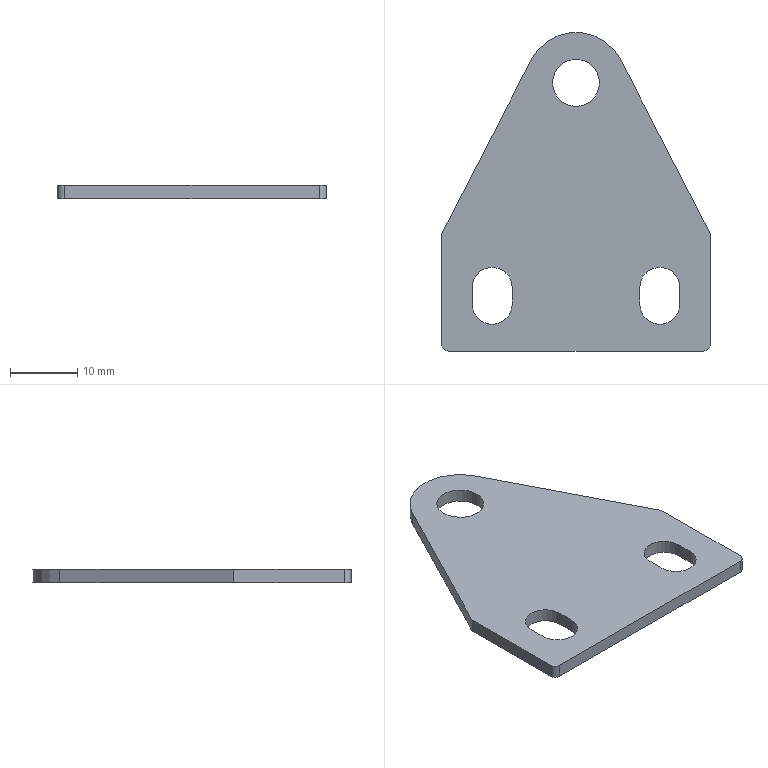Part | STEP file | LE-MX-A-P1_PN_0007 | 1 solid | 20 faces | box 40 x 47.5 x 2 mm | volume 2610 mm3 | plane 11 | cylinder 9 | commonest cylinder face diameters 6 x4 2 x2 7 x2 15 x1
STEP:
#1=CARTESIAN_POINT('',(-3.5,40.,2.));
#2=VERTEX_POINT('',#1);
#3=CARTESIAN_POINT('',(3.5,40.,2.));
#4=VERTEX_POINT('',#3);
#5=CARTESIAN_POINT('',(0.,40.,2.));
#6=DIRECTION('',(0.,0.,1.));
#7=DIRECTION('',(-1.,0.,0.));
#8=AXIS2_PLACEMENT_3D('',#5,#6,#7);
#9=CIRCLE('',#8,3.5);
#10=EDGE_CURVE('',#2,#4,#9,.T.);
#11=ORIENTED_EDGE('',*,*,#10,.T.);
#12=CARTESIAN_POINT('',(3.5,40.,0.));
#13=VERTEX_POINT('',#12);
#14=CARTESIAN_POINT('',(3.5,40.,2.));
#15=DIRECTION('',(0.,0.,-1.));
#16=VECTOR('',#15,1000.);
#17=LINE('',#14,#16);
#18=EDGE_CURVE('',#4,#13,#17,.T.);
#19=ORIENTED_EDGE('',*,*,#18,.T.);
#20=CARTESIAN_POINT('',(-3.5,40.,0.));
#21=VERTEX_POINT('',#20);
#22=CARTESIAN_POINT('',(0.,40.,0.));
#23=DIRECTION('',(0.,0.,1.));
#24=DIRECTION('',(-1.,0.,0.));
#25=AXIS2_PLACEMENT_3D('',#22,#23,#24);
#26=CIRCLE('',#25,3.5);
#27=EDGE_CURVE('',#21,#13,#26,.T.);
#28=ORIENTED_EDGE('',*,*,#27,.F.);
#29=CARTESIAN_POINT('',(-3.5,40.,2.));
#30=DIRECTION('',(0.,0.,-1.));
#31=VECTOR('',#30,1000.);
#32=LINE('',#29,#31);
#33=EDGE_CURVE('',#2,#21,#32,.T.);
#34=ORIENTED_EDGE('',*,*,#33,.F.);
#35=EDGE_LOOP('',(#11,#19,#28,#34));
#36=FACE_OUTER_BOUND('',#35,.T.);
#37=CARTESIAN_POINT('',(0.,40.,2.));
#38=DIRECTION('',(0.,0.,-1.));
#39=DIRECTION('',(-1.,0.,0.));
#40=AXIS2_PLACEMENT_3D('',#37,#38,#39);
#41=CYLINDRICAL_SURFACE('',#40,3.5);
#42=ADVANCED_FACE('',(#36),#41,.F.);
#43=CARTESIAN_POINT('',(-20.,17.5,2.));
#44=VERTEX_POINT('',#43);
#45=CARTESIAN_POINT('',(-6.67,43.429,2.));
#46=VERTEX_POINT('',#45);
#47=CARTESIAN_POINT('',(-20.,17.5,2.));
#48=DIRECTION('',(0.4572,0.8894,0.));
#49=VECTOR('',#48,1000.);
#50=LINE('',#47,#49);
#51=EDGE_CURVE('',#44,#46,#50,.T.);
#52=ORIENTED_EDGE('',*,*,#51,.F.);
#53=CARTESIAN_POINT('',(-20.,1.,2.));
#54=VERTEX_POINT('',#53);
#55=CARTESIAN_POINT('',(-20.,40.,2.));
#56=DIRECTION('',(0.,1.,0.));
#57=VECTOR('',#56,1000.);
#58=LINE('',#55,#57);
#59=EDGE_CURVE('',#54,#44,#58,.T.);
#60=ORIENTED_EDGE('',*,*,#59,.F.);
#61=CARTESIAN_POINT('',(-19.,0.,2.));
#62=VERTEX_POINT('',#61);
#63=CARTESIAN_POINT('',(-19.,1.,2.));
#64=DIRECTION('',(0.,0.,-1.));
#65=DIRECTION('',(-1.,0.,0.));
#66=AXIS2_PLACEMENT_3D('',#63,#64,#65);
#67=CIRCLE('',#66,1.);
#68=EDGE_CURVE('',#62,#54,#67,.T.);
#69=ORIENTED_EDGE('',*,*,#68,.F.);
#70=CARTESIAN_POINT('',(19.,0.,2.));
#71=VERTEX_POINT('',#70);
#72=CARTESIAN_POINT('',(0.,0.,2.));
#73=DIRECTION('',(-1.,0.,0.));
#74=VECTOR('',#73,1000.);
#75=LINE('',#72,#74);
#76=EDGE_CURVE('',#71,#62,#75,.T.);
#77=ORIENTED_EDGE('',*,*,#76,.F.);
#78=CARTESIAN_POINT('',(20.,1.,2.));
#79=VERTEX_POINT('',#78);
#80=CARTESIAN_POINT('',(19.,1.,2.));
#81=DIRECTION('',(0.,0.,-1.));
#82=DIRECTION('',(-1.,0.,0.));
#83=AXIS2_PLACEMENT_3D('',#80,#81,#82);
#84=CIRCLE('',#83,1.);
#85=EDGE_CURVE('',#79,#71,#84,.T.);
#86=ORIENTED_EDGE('',*,*,#85,.F.);
#87=CARTESIAN_POINT('',(20.,17.5,2.));
#88=VERTEX_POINT('',#87);
#89=CARTESIAN_POINT('',(20.,40.,2.));
#90=DIRECTION('',(0.,-1.,0.));
#91=VECTOR('',#90,1000.);
#92=LINE('',#89,#91);
#93=EDGE_CURVE('',#88,#79,#92,.T.);
#94=ORIENTED_EDGE('',*,*,#93,.F.);
#95=CARTESIAN_POINT('',(6.67,43.429,2.));
#96=VERTEX_POINT('',#95);
#97=CARTESIAN_POINT('',(6.67,43.429,2.));
#98=DIRECTION('',(0.4572,-0.8894,0.));
#99=VECTOR('',#98,1000.);
#100=LINE('',#97,#99);
#101=EDGE_CURVE('',#96,#88,#100,.T.);
#102=ORIENTED_EDGE('',*,*,#101,.F.);
#103=CARTESIAN_POINT('',(0.,40.,2.));
#104=DIRECTION('',(0.,0.,-1.));
#105=DIRECTION('',(-1.,0.,0.));
#106=AXIS2_PLACEMENT_3D('',#103,#104,#105);
#107=CIRCLE('',#106,7.5);
#108=EDGE_CURVE('',#46,#96,#107,.T.);
#109=ORIENTED_EDGE('',*,*,#108,.F.);
#110=EDGE_LOOP('',(#52,#60,#69,#77,#86,#94,#102,#109));
#111=FACE_OUTER_BOUND('',#110,.T.);
#112=CARTESIAN_POINT('',(15.5,9.5,2.));
#113=VERTEX_POINT('',#112);
#114=CARTESIAN_POINT('',(9.5,9.5,2.));
#115=VERTEX_POINT('',#114);
#116=CARTESIAN_POINT('',(12.5,9.5,2.));
#117=DIRECTION('',(0.,0.,1.));
#118=DIRECTION('',(-1.,0.,0.));
#119=AXIS2_PLACEMENT_3D('',#116,#117,#118);
#120=CIRCLE('',#119,3.);
#121=EDGE_CURVE('',#113,#115,#120,.T.);
#122=ORIENTED_EDGE('',*,*,#121,.F.);
#123=CARTESIAN_POINT('',(15.5,7.,2.));
#124=VERTEX_POINT('',#123);
#125=CARTESIAN_POINT('',(15.5,40.,2.));
#126=DIRECTION('',(0.,1.,0.));
#127=VECTOR('',#126,1000.);
#128=LINE('',#125,#127);
#129=EDGE_CURVE('',#124,#113,#128,.T.);
#130=ORIENTED_EDGE('',*,*,#129,.F.);
#131=CARTESIAN_POINT('',(9.5,7.,2.));
#132=VERTEX_POINT('',#131);
#133=CARTESIAN_POINT('',(12.5,7.,2.));
#134=DIRECTION('',(0.,0.,1.));
#135=DIRECTION('',(-1.,0.,0.));
#136=AXIS2_PLACEMENT_3D('',#133,#134,#135);
#137=CIRCLE('',#136,3.);
#138=EDGE_CURVE('',#132,#124,#137,.T.);
#139=ORIENTED_EDGE('',*,*,#138,.F.);
#140=CARTESIAN_POINT('',(9.5,40.,2.));
#141=DIRECTION('',(0.,-1.,0.));
#142=VECTOR('',#141,1000.);
#143=LINE('',#140,#142);
#144=EDGE_CURVE('',#115,#132,#143,.T.);
#145=ORIENTED_EDGE('',*,*,#144,.F.);
#146=EDGE_LOOP('',(#122,#130,#139,#145));
#147=FACE_BOUND('',#146,.T.);
#148=ORIENTED_EDGE('',*,*,#10,.F.);
#149=CARTESIAN_POINT('',(0.,40.,2.));
#150=DIRECTION('',(0.,0.,1.));
#151=DIRECTION('',(-1.,0.,0.));
#152=AXIS2_PLACEMENT_3D('',#149,#150,#151);
#153=CIRCLE('',#152,3.5);
#154=EDGE_CURVE('',#4,#2,#153,.T.);
#155=ORIENTED_EDGE('',*,*,#154,.F.);
#156=EDGE_LOOP('',(#148,#155));
#157=FACE_BOUND('',#156,.T.);
#158=CARTESIAN_POINT('',(-9.5,9.5,2.));
#159=VERTEX_POINT('',#158);
#160=CARTESIAN_POINT('',(-15.5,9.5,2.));
#161=VERTEX_POINT('',#160);
#162=CARTESIAN_POINT('',(-12.5,9.5,2.));
#163=DIRECTION('',(0.,0.,1.));
#164=DIRECTION('',(-1.,0.,0.));
#165=AXIS2_PLACEMENT_3D('',#162,#163,#164);
#166=CIRCLE('',#165,3.);
#167=EDGE_CURVE('',#159,#161,#166,.T.);
#168=ORIENTED_EDGE('',*,*,#167,.F.);
#169=CARTESIAN_POINT('',(-9.5,7.,2.));
#170=VERTEX_POINT('',#169);
#171=CARTESIAN_POINT('',(-9.5,40.,2.));
#172=DIRECTION('',(0.,1.,0.));
#173=VECTOR('',#172,1000.);
#174=LINE('',#171,#173);
#175=EDGE_CURVE('',#170,#159,#174,.T.);
#176=ORIENTED_EDGE('',*,*,#175,.F.);
#177=CARTESIAN_POINT('',(-15.5,7.,2.));
#178=VERTEX_POINT('',#177);
#179=CARTESIAN_POINT('',(-12.5,7.,2.));
#180=DIRECTION('',(0.,0.,1.));
#181=DIRECTION('',(-1.,0.,0.));
#182=AXIS2_PLACEMENT_3D('',#179,#180,#181);
#183=CIRCLE('',#182,3.);
#184=EDGE_CURVE('',#178,#170,#183,.T.);
#185=ORIENTED_EDGE('',*,*,#184,.F.);
#186=CARTESIAN_POINT('',(-15.5,40.,2.));
#187=DIRECTION('',(0.,-1.,0.));
#188=VECTOR('',#187,1000.);
#189=LINE('',#186,#188);
#190=EDGE_CURVE('',#161,#178,#189,.T.);
#191=ORIENTED_EDGE('',*,*,#190,.F.);
#192=EDGE_LOOP('',(#168,#176,#185,#191));
#193=FACE_BOUND('',#192,.T.);
#194=CARTESIAN_POINT('',(0.,40.,2.));
#195=DIRECTION('',(0.,0.,-1.));
#196=DIRECTION('',(-1.,0.,0.));
#197=AXIS2_PLACEMENT_3D('',#194,#195,#196);
#198=PLANE('',#197);
#199=ADVANCED_FACE('',(#111,#147,#157,#193),#198,.F.);
#200=ORIENTED_EDGE('',*,*,#108,.T.);
#201=CARTESIAN_POINT('',(6.67,43.429,0.));
#202=VERTEX_POINT('',#201);
#203=CARTESIAN_POINT('',(6.67,43.429,2.));
#204=DIRECTION('',(0.,0.,-1.));
#205=VECTOR('',#204,1000.);
#206=LINE('',#203,#205);
#207=EDGE_CURVE('',#96,#202,#206,.T.);
#208=ORIENTED_EDGE('',*,*,#207,.T.);
#209=CARTESIAN_POINT('',(-6.67,43.429,0.));
#210=VERTEX_POINT('',#209);
#211=CARTESIAN_POINT('',(0.,40.,0.));
#212=DIRECTION('',(0.,0.,1.));
#213=DIRECTION('',(-1.,0.,0.));
#214=AXIS2_PLACEMENT_3D('',#211,#212,#213);
#215=CIRCLE('',#214,7.5);
#216=EDGE_CURVE('',#202,#210,#215,.T.);
#217=ORIENTED_EDGE('',*,*,#216,.T.);
#218=CARTESIAN_POINT('',(-6.67,43.429,2.));
#219=DIRECTION('',(0.,0.,1.));
#220=VECTOR('',#219,1000.);
#221=LINE('',#218,#220);
#222=EDGE_CURVE('',#210,#46,#221,.T.);
#223=ORIENTED_EDGE('',*,*,#222,.T.);
#224=EDGE_LOOP('',(#200,#208,#217,#223));
#225=FACE_OUTER_BOUND('',#224,.T.);
#226=CARTESIAN_POINT('',(0.,40.,2.));
#227=DIRECTION('',(0.,0.,-1.));
#228=DIRECTION('',(-1.,0.,0.));
#229=AXIS2_PLACEMENT_3D('',#226,#227,#228);
#230=CYLINDRICAL_SURFACE('',#229,7.5);
#231=ADVANCED_FACE('',(#225),#230,.T.);
#232=ORIENTED_EDGE('',*,*,#51,.T.);
#233=ORIENTED_EDGE('',*,*,#222,.F.);
#234=CARTESIAN_POINT('',(-20.,17.5,0.));
#235=VERTEX_POINT('',#234);
#236=CARTESIAN_POINT('',(-20.,17.5,0.));
#237=DIRECTION('',(-0.4572,-0.8894,0.));
#238=VECTOR('',#237,1000.);
#239=LINE('',#236,#238);
#240=EDGE_CURVE('',#210,#235,#239,.T.);
#241=ORIENTED_EDGE('',*,*,#240,.T.);
#242=CARTESIAN_POINT('',(-20.,17.5,2.));
#243=DIRECTION('',(0.,0.,1.));
#244=VECTOR('',#243,1000.);
#245=LINE('',#242,#244);
#246=EDGE_CURVE('',#235,#44,#245,.T.);
#247=ORIENTED_EDGE('',*,*,#246,.T.);
#248=EDGE_LOOP('',(#232,#233,#241,#247));
#249=FACE_OUTER_BOUND('',#248,.T.);
#250=CARTESIAN_POINT('',(-20.,17.5,2.));
#251=DIRECTION('',(-0.8894,0.4572,0.));
#252=DIRECTION('',(-0.4572,-0.8894,0.));
#253=AXIS2_PLACEMENT_3D('',#250,#251,#252);
#254=PLANE('',#253);
#255=ADVANCED_FACE('',(#249),#254,.T.);
#256=ORIENTED_EDGE('',*,*,#59,.T.);
#257=ORIENTED_EDGE('',*,*,#246,.F.);
#258=CARTESIAN_POINT('',(-20.,1.,0.));
#259=VERTEX_POINT('',#258);
#260=CARTESIAN_POINT('',(-20.,1.,0.));
#261=DIRECTION('',(0.,-1.,0.));
#262=VECTOR('',#261,1000.);
#263=LINE('',#260,#262);
#264=EDGE_CURVE('',#235,#259,#263,.T.);
#265=ORIENTED_EDGE('',*,*,#264,.T.);
#266=CARTESIAN_POINT('',(-20.,1.,2.));
#267=DIRECTION('',(0.,0.,1.));
#268=VECTOR('',#267,1000.);
#269=LINE('',#266,#268);
#270=EDGE_CURVE('',#259,#54,#269,.T.);
#271=ORIENTED_EDGE('',*,*,#270,.T.);
#272=EDGE_LOOP('',(#256,#257,#265,#271));
#273=FACE_OUTER_BOUND('',#272,.T.);
#274=CARTESIAN_POINT('',(-20.,1.,2.));
#275=DIRECTION('',(-1.,0.,0.));
#276=DIRECTION('',(0.,0.,1.));
#277=AXIS2_PLACEMENT_3D('',#274,#275,#276);
#278=PLANE('',#277);
#279=ADVANCED_FACE('',(#273),#278,.T.);
#280=ORIENTED_EDGE('',*,*,#76,.T.);
#281=CARTESIAN_POINT('',(-19.,0.,0.));
#282=VERTEX_POINT('',#281);
#283=CARTESIAN_POINT('',(-19.,0.,2.));
#284=DIRECTION('',(0.,0.,-1.));
#285=VECTOR('',#284,1000.);
#286=LINE('',#283,#285);
#287=EDGE_CURVE('',#62,#282,#286,.T.);
#288=ORIENTED_EDGE('',*,*,#287,.T.);
#289=CARTESIAN_POINT('',(19.,0.,0.));
#290=VERTEX_POINT('',#289);
#291=CARTESIAN_POINT('',(19.,0.,0.));
#292=DIRECTION('',(1.,0.,0.));
#293=VECTOR('',#292,1000.);
#294=LINE('',#291,#293);
#295=EDGE_CURVE('',#282,#290,#294,.T.);
#296=ORIENTED_EDGE('',*,*,#295,.T.);
#297=CARTESIAN_POINT('',(19.,0.,2.));
#298=DIRECTION('',(0.,0.,1.));
#299=VECTOR('',#298,1000.);
#300=LINE('',#297,#299);
#301=EDGE_CURVE('',#290,#71,#300,.T.);
#302=ORIENTED_EDGE('',*,*,#301,.T.);
#303=EDGE_LOOP('',(#280,#288,#296,#302));
#304=FACE_OUTER_BOUND('',#303,.T.);
#305=CARTESIAN_POINT('',(19.,0.,2.));
#306=DIRECTION('',(0.,-1.,0.));
#307=DIRECTION('',(1.,0.,0.));
#308=AXIS2_PLACEMENT_3D('',#305,#306,#307);
#309=PLANE('',#308);
#310=ADVANCED_FACE('',(#304),#309,.T.);
#311=ORIENTED_EDGE('',*,*,#93,.T.);
#312=CARTESIAN_POINT('',(20.,1.,0.));
#313=VERTEX_POINT('',#312);
#314=CARTESIAN_POINT('',(20.,1.,2.));
#315=DIRECTION('',(0.,0.,-1.));
#316=VECTOR('',#315,1000.);
#317=LINE('',#314,#316);
#318=EDGE_CURVE('',#79,#313,#317,.T.);
#319=ORIENTED_EDGE('',*,*,#318,.T.);
#320=CARTESIAN_POINT('',(20.,17.5,0.));
#321=VERTEX_POINT('',#320);
#322=CARTESIAN_POINT('',(20.,17.5,0.));
#323=DIRECTION('',(0.,1.,0.));
#324=VECTOR('',#323,1000.);
#325=LINE('',#322,#324);
#326=EDGE_CURVE('',#313,#321,#325,.T.);
#327=ORIENTED_EDGE('',*,*,#326,.T.);
#328=CARTESIAN_POINT('',(20.,17.5,2.));
#329=DIRECTION('',(0.,0.,1.));
#330=VECTOR('',#329,1000.);
#331=LINE('',#328,#330);
#332=EDGE_CURVE('',#321,#88,#331,.T.);
#333=ORIENTED_EDGE('',*,*,#332,.T.);
#334=EDGE_LOOP('',(#311,#319,#327,#333));
#335=FACE_OUTER_BOUND('',#334,.T.);
#336=CARTESIAN_POINT('',(20.,17.5,2.));
#337=DIRECTION('',(1.,0.,0.));
#338=DIRECTION('',(0.,0.,-1.));
#339=AXIS2_PLACEMENT_3D('',#336,#337,#338);
#340=PLANE('',#339);
#341=ADVANCED_FACE('',(#335),#340,.T.);
#342=ORIENTED_EDGE('',*,*,#101,.T.);
#343=ORIENTED_EDGE('',*,*,#332,.F.);
#344=CARTESIAN_POINT('',(6.67,43.429,0.));
#345=DIRECTION('',(-0.4572,0.8894,0.));
#346=VECTOR('',#345,1000.);
#347=LINE('',#344,#346);
#348=EDGE_CURVE('',#321,#202,#347,.T.);
#349=ORIENTED_EDGE('',*,*,#348,.T.);
#350=ORIENTED_EDGE('',*,*,#207,.F.);
#351=EDGE_LOOP('',(#342,#343,#349,#350));
#352=FACE_OUTER_BOUND('',#351,.T.);
#353=CARTESIAN_POINT('',(6.67,43.429,2.));
#354=DIRECTION('',(0.8894,0.4572,0.));
#355=DIRECTION('',(-0.4572,0.8894,0.));
#356=AXIS2_PLACEMENT_3D('',#353,#354,#355);
#357=PLANE('',#356);
#358=ADVANCED_FACE('',(#352),#357,.T.);
#359=CARTESIAN_POINT('',(9.5,9.5,0.));
#360=VERTEX_POINT('',#359);
#361=CARTESIAN_POINT('',(9.5,9.5,2.));
#362=DIRECTION('',(0.,0.,-1.));
#363=VECTOR('',#362,1000.);
#364=LINE('',#361,#363);
#365=EDGE_CURVE('',#115,#360,#364,.T.);
#366=ORIENTED_EDGE('',*,*,#365,.F.);
#367=ORIENTED_EDGE('',*,*,#144,.T.);
#368=CARTESIAN_POINT('',(9.5,7.,0.));
#369=VERTEX_POINT('',#368);
#370=CARTESIAN_POINT('',(9.5,7.,2.));
#371=DIRECTION('',(0.,0.,1.));
#372=VECTOR('',#371,1000.);
#373=LINE('',#370,#372);
#374=EDGE_CURVE('',#369,#132,#373,.T.);
#375=ORIENTED_EDGE('',*,*,#374,.F.);
#376=CARTESIAN_POINT('',(9.5,9.5,0.));
#377=DIRECTION('',(0.,-1.,0.));
#378=VECTOR('',#377,1000.);
#379=LINE('',#376,#378);
#380=EDGE_CURVE('',#360,#369,#379,.T.);
#381=ORIENTED_EDGE('',*,*,#380,.F.);
#382=EDGE_LOOP('',(#366,#367,#375,#381));
#383=FACE_OUTER_BOUND('',#382,.T.);
#384=CARTESIAN_POINT('',(9.5,9.5,2.));
#385=DIRECTION('',(-1.,0.,0.));
#386=DIRECTION('',(0.,-1.,0.));
#387=AXIS2_PLACEMENT_3D('',#384,#385,#386);
#388=PLANE('',#387);
#389=ADVANCED_FACE('',(#383),#388,.F.);
#390=CARTESIAN_POINT('',(15.5,9.5,0.));
#391=VERTEX_POINT('',#390);
#392=CARTESIAN_POINT('',(15.5,9.5,2.));
#393=DIRECTION('',(0.,0.,-1.));
#394=VECTOR('',#393,1000.);
#395=LINE('',#392,#394);
#396=EDGE_CURVE('',#113,#391,#395,.T.);
#397=ORIENTED_EDGE('',*,*,#396,.F.);
#398=ORIENTED_EDGE('',*,*,#121,.T.);
#399=ORIENTED_EDGE('',*,*,#365,.T.);
#400=CARTESIAN_POINT('',(12.5,9.5,0.));
#401=DIRECTION('',(0.,0.,1.));
#402=DIRECTION('',(-1.,0.,0.));
#403=AXIS2_PLACEMENT_3D('',#400,#401,#402);
#404=CIRCLE('',#403,3.);
#405=EDGE_CURVE('',#391,#360,#404,.T.);
#406=ORIENTED_EDGE('',*,*,#405,.F.);
#407=EDGE_LOOP('',(#397,#398,#399,#406));
#408=FACE_OUTER_BOUND('',#407,.T.);
#409=CARTESIAN_POINT('',(12.5,9.5,2.));
#410=DIRECTION('',(0.,0.,-1.));
#411=DIRECTION('',(-1.,0.,0.));
#412=AXIS2_PLACEMENT_3D('',#409,#410,#411);
#413=CYLINDRICAL_SURFACE('',#412,3.);
#414=ADVANCED_FACE('',(#408),#413,.F.);
#415=CARTESIAN_POINT('',(15.5,7.,0.));
#416=VERTEX_POINT('',#415);
#417=CARTESIAN_POINT('',(15.5,7.,2.));
#418=DIRECTION('',(0.,0.,-1.));
#419=VECTOR('',#418,1000.);
#420=LINE('',#417,#419);
#421=EDGE_CURVE('',#124,#416,#420,.T.);
#422=ORIENTED_EDGE('',*,*,#421,.F.);
#423=ORIENTED_EDGE('',*,*,#129,.T.);
#424=ORIENTED_EDGE('',*,*,#396,.T.);
#425=CARTESIAN_POINT('',(15.5,7.,0.));
#426=DIRECTION('',(0.,1.,0.));
#427=VECTOR('',#426,1000.);
#428=LINE('',#425,#427);
#429=EDGE_CURVE('',#416,#391,#428,.T.);
#430=ORIENTED_EDGE('',*,*,#429,.F.);
#431=EDGE_LOOP('',(#422,#423,#424,#430));
#432=FACE_OUTER_BOUND('',#431,.T.);
#433=CARTESIAN_POINT('',(15.5,7.,2.));
#434=DIRECTION('',(1.,0.,0.));
#435=DIRECTION('',(0.,1.,0.));
#436=AXIS2_PLACEMENT_3D('',#433,#434,#435);
#437=PLANE('',#436);
#438=ADVANCED_FACE('',(#432),#437,.F.);
#439=ORIENTED_EDGE('',*,*,#374,.T.);
#440=ORIENTED_EDGE('',*,*,#138,.T.);
#441=ORIENTED_EDGE('',*,*,#421,.T.);
#442=CARTESIAN_POINT('',(12.5,7.,0.));
#443=DIRECTION('',(0.,0.,1.));
#444=DIRECTION('',(-1.,0.,0.));
#445=AXIS2_PLACEMENT_3D('',#442,#443,#444);
#446=CIRCLE('',#445,3.);
#447=EDGE_CURVE('',#369,#416,#446,.T.);
#448=ORIENTED_EDGE('',*,*,#447,.F.);
#449=EDGE_LOOP('',(#439,#440,#441,#448));
#450=FACE_OUTER_BOUND('',#449,.T.);
#451=CARTESIAN_POINT('',(12.5,7.,2.));
#452=DIRECTION('',(0.,0.,-1.));
#453=DIRECTION('',(-1.,0.,0.));
#454=AXIS2_PLACEMENT_3D('',#451,#452,#453);
#455=CYLINDRICAL_SURFACE('',#454,3.);
#456=ADVANCED_FACE('',(#450),#455,.F.);
#457=ORIENTED_EDGE('',*,*,#18,.F.);
#458=ORIENTED_EDGE('',*,*,#154,.T.);
#459=ORIENTED_EDGE('',*,*,#33,.T.);
#460=CARTESIAN_POINT('',(0.,40.,0.));
#461=DIRECTION('',(0.,0.,1.));
#462=DIRECTION('',(-1.,0.,0.));
#463=AXIS2_PLACEMENT_3D('',#460,#461,#462);
#464=CIRCLE('',#463,3.5);
#465=EDGE_CURVE('',#13,#21,#464,.T.);
#466=ORIENTED_EDGE('',*,*,#465,.F.);
#467=EDGE_LOOP('',(#457,#458,#459,#466));
#468=FACE_OUTER_BOUND('',#467,.T.);
#469=CARTESIAN_POINT('',(0.,40.,2.));
#470=DIRECTION('',(0.,0.,-1.));
#471=DIRECTION('',(-1.,0.,0.));
#472=AXIS2_PLACEMENT_3D('',#469,#470,#471);
#473=CYLINDRICAL_SURFACE('',#472,3.5);
#474=ADVANCED_FACE('',(#468),#473,.F.);
#475=CARTESIAN_POINT('',(-15.5,9.5,0.));
#476=VERTEX_POINT('',#475);
#477=CARTESIAN_POINT('',(-15.5,9.5,2.));
#478=DIRECTION('',(0.,0.,-1.));
#479=VECTOR('',#478,1000.);
#480=LINE('',#477,#479);
#481=EDGE_CURVE('',#161,#476,#480,.T.);
#482=ORIENTED_EDGE('',*,*,#481,.F.);
#483=ORIENTED_EDGE('',*,*,#190,.T.);
#484=CARTESIAN_POINT('',(-15.5,7.,0.));
#485=VERTEX_POINT('',#484);
#486=CARTESIAN_POINT('',(-15.5,7.,2.));
#487=DIRECTION('',(0.,0.,1.));
#488=VECTOR('',#487,1000.);
#489=LINE('',#486,#488);
#490=EDGE_CURVE('',#485,#178,#489,.T.);
#491=ORIENTED_EDGE('',*,*,#490,.F.);
#492=CARTESIAN_POINT('',(-15.5,9.5,0.));
#493=DIRECTION('',(0.,-1.,0.));
#494=VECTOR('',#493,1000.);
#495=LINE('',#492,#494);
#496=EDGE_CURVE('',#476,#485,#495,.T.);
#497=ORIENTED_EDGE('',*,*,#496,.F.);
#498=EDGE_LOOP('',(#482,#483,#491,#497));
#499=FACE_OUTER_BOUND('',#498,.T.);
#500=CARTESIAN_POINT('',(-15.5,9.5,2.));
#501=DIRECTION('',(-1.,0.,0.));
#502=DIRECTION('',(0.,-1.,0.));
#503=AXIS2_PLACEMENT_3D('',#500,#501,#502);
#504=PLANE('',#503);
#505=ADVANCED_FACE('',(#499),#504,.F.);
#506=CARTESIAN_POINT('',(-9.5,9.5,0.));
#507=VERTEX_POINT('',#506);
#508=CARTESIAN_POINT('',(-9.5,9.5,2.));
#509=DIRECTION('',(0.,0.,-1.));
#510=VECTOR('',#509,1000.);
#511=LINE('',#508,#510);
#512=EDGE_CURVE('',#159,#507,#511,.T.);
#513=ORIENTED_EDGE('',*,*,#512,.F.);
#514=ORIENTED_EDGE('',*,*,#167,.T.);
#515=ORIENTED_EDGE('',*,*,#481,.T.);
#516=CARTESIAN_POINT('',(-12.5,9.5,0.));
#517=DIRECTION('',(0.,0.,1.));
#518=DIRECTION('',(-1.,0.,0.));
#519=AXIS2_PLACEMENT_3D('',#516,#517,#518);
#520=CIRCLE('',#519,3.);
#521=EDGE_CURVE('',#507,#476,#520,.T.);
#522=ORIENTED_EDGE('',*,*,#521,.F.);
#523=EDGE_LOOP('',(#513,#514,#515,#522));
#524=FACE_OUTER_BOUND('',#523,.T.);
#525=CARTESIAN_POINT('',(-12.5,9.5,2.));
#526=DIRECTION('',(0.,0.,-1.));
#527=DIRECTION('',(-1.,0.,0.));
#528=AXIS2_PLACEMENT_3D('',#525,#526,#527);
#529=CYLINDRICAL_SURFACE('',#528,3.);
#530=ADVANCED_FACE('',(#524),#529,.F.);
#531=CARTESIAN_POINT('',(-9.5,7.,0.));
#532=VERTEX_POINT('',#531);
#533=CARTESIAN_POINT('',(-9.5,7.,2.));
#534=DIRECTION('',(0.,0.,-1.));
#535=VECTOR('',#534,1000.);
#536=LINE('',#533,#535);
#537=EDGE_CURVE('',#170,#532,#536,.T.);
#538=ORIENTED_EDGE('',*,*,#537,.F.);
#539=ORIENTED_EDGE('',*,*,#175,.T.);
#540=ORIENTED_EDGE('',*,*,#512,.T.);
#541=CARTESIAN_POINT('',(-9.5,7.,0.));
#542=DIRECTION('',(0.,1.,0.));
#543=VECTOR('',#542,1000.);
#544=LINE('',#541,#543);
#545=EDGE_CURVE('',#532,#507,#544,.T.);
#546=ORIENTED_EDGE('',*,*,#545,.F.);
#547=EDGE_LOOP('',(#538,#539,#540,#546));
#548=FACE_OUTER_BOUND('',#547,.T.);
#549=CARTESIAN_POINT('',(-9.5,7.,2.));
#550=DIRECTION('',(1.,0.,0.));
#551=DIRECTION('',(0.,0.,-1.));
#552=AXIS2_PLACEMENT_3D('',#549,#550,#551);
#553=PLANE('',#552);
#554=ADVANCED_FACE('',(#548),#553,.F.);
#555=ORIENTED_EDGE('',*,*,#490,.T.);
#556=ORIENTED_EDGE('',*,*,#184,.T.);
#557=ORIENTED_EDGE('',*,*,#537,.T.);
#558=CARTESIAN_POINT('',(-12.5,7.,0.));
#559=DIRECTION('',(0.,0.,1.));
#560=DIRECTION('',(-1.,0.,0.));
#561=AXIS2_PLACEMENT_3D('',#558,#559,#560);
#562=CIRCLE('',#561,3.);
#563=EDGE_CURVE('',#485,#532,#562,.T.);
#564=ORIENTED_EDGE('',*,*,#563,.F.);
#565=EDGE_LOOP('',(#555,#556,#557,#564));
#566=FACE_OUTER_BOUND('',#565,.T.);
#567=CARTESIAN_POINT('',(-12.5,7.,2.));
#568=DIRECTION('',(0.,0.,-1.));
#569=DIRECTION('',(-1.,0.,0.));
#570=AXIS2_PLACEMENT_3D('',#567,#568,#569);
#571=CYLINDRICAL_SURFACE('',#570,3.);
#572=ADVANCED_FACE('',(#566),#571,.F.);
#573=ORIENTED_EDGE('',*,*,#264,.F.);
#574=ORIENTED_EDGE('',*,*,#240,.F.);
#575=ORIENTED_EDGE('',*,*,#216,.F.);
#576=ORIENTED_EDGE('',*,*,#348,.F.);
#577=ORIENTED_EDGE('',*,*,#326,.F.);
#578=CARTESIAN_POINT('',(19.,1.,0.));
#579=DIRECTION('',(0.,0.,-1.));
#580=DIRECTION('',(-1.,0.,0.));
#581=AXIS2_PLACEMENT_3D('',#578,#579,#580);
#582=CIRCLE('',#581,1.);
#583=EDGE_CURVE('',#313,#290,#582,.T.);
#584=ORIENTED_EDGE('',*,*,#583,.T.);
#585=ORIENTED_EDGE('',*,*,#295,.F.);
#586=CARTESIAN_POINT('',(-19.,1.,0.));
#587=DIRECTION('',(0.,0.,-1.));
#588=DIRECTION('',(-1.,0.,0.));
#589=AXIS2_PLACEMENT_3D('',#586,#587,#588);
#590=CIRCLE('',#589,1.);
#591=EDGE_CURVE('',#282,#259,#590,.T.);
#592=ORIENTED_EDGE('',*,*,#591,.T.);
#593=EDGE_LOOP('',(#573,#574,#575,#576,#577,#584,#585,#592));
#594=FACE_OUTER_BOUND('',#593,.T.);
#595=ORIENTED_EDGE('',*,*,#447,.T.);
#596=ORIENTED_EDGE('',*,*,#429,.T.);
#597=ORIENTED_EDGE('',*,*,#405,.T.);
#598=ORIENTED_EDGE('',*,*,#380,.T.);
#599=EDGE_LOOP('',(#595,#596,#597,#598));
#600=FACE_BOUND('',#599,.T.);
#601=ORIENTED_EDGE('',*,*,#27,.T.);
#602=ORIENTED_EDGE('',*,*,#465,.T.);
#603=EDGE_LOOP('',(#601,#602));
#604=FACE_BOUND('',#603,.T.);
#605=ORIENTED_EDGE('',*,*,#563,.T.);
#606=ORIENTED_EDGE('',*,*,#545,.T.);
#607=ORIENTED_EDGE('',*,*,#521,.T.);
#608=ORIENTED_EDGE('',*,*,#496,.T.);
#609=EDGE_LOOP('',(#605,#606,#607,#608));
#610=FACE_BOUND('',#609,.T.);
#611=CARTESIAN_POINT('',(0.,40.,0.));
#612=DIRECTION('',(0.,0.,-1.));
#613=DIRECTION('',(-1.,0.,0.));
#614=AXIS2_PLACEMENT_3D('',#611,#612,#613);
#615=PLANE('',#614);
#616=ADVANCED_FACE('',(#594,#600,#604,#610),#615,.T.);
#617=ORIENTED_EDGE('',*,*,#68,.T.);
#618=ORIENTED_EDGE('',*,*,#270,.F.);
#619=ORIENTED_EDGE('',*,*,#591,.F.);
#620=ORIENTED_EDGE('',*,*,#287,.F.);
#621=EDGE_LOOP('',(#617,#618,#619,#620));
#622=FACE_OUTER_BOUND('',#621,.T.);
#623=CARTESIAN_POINT('',(-19.,1.,2.));
#624=DIRECTION('',(0.,0.,-1.));
#625=DIRECTION('',(-1.,0.,0.));
#626=AXIS2_PLACEMENT_3D('',#623,#624,#625);
#627=CYLINDRICAL_SURFACE('',#626,1.);
#628=ADVANCED_FACE('',(#622),#627,.T.);
#629=ORIENTED_EDGE('',*,*,#85,.T.);
#630=ORIENTED_EDGE('',*,*,#301,.F.);
#631=ORIENTED_EDGE('',*,*,#583,.F.);
#632=ORIENTED_EDGE('',*,*,#318,.F.);
#633=EDGE_LOOP('',(#629,#630,#631,#632));
#634=FACE_OUTER_BOUND('',#633,.T.);
#635=CARTESIAN_POINT('',(19.,1.,2.));
#636=DIRECTION('',(0.,0.,-1.));
#637=DIRECTION('',(-1.,0.,0.));
#638=AXIS2_PLACEMENT_3D('',#635,#636,#637);
#639=CYLINDRICAL_SURFACE('',#638,1.);
#640=ADVANCED_FACE('',(#634),#639,.T.);
#641=CLOSED_SHELL('',(#42,#199,#231,#255,#279,#310,#341,#358,#389,#414,#438,#456,#474,#505,#530,#554,#572,#616,#628,#640));
#642=MANIFOLD_SOLID_BREP('',#641);
#643=CARTESIAN_POINT('',(0.,0.,0.));
#644=DIRECTION('',(0.,0.,1.));
#645=DIRECTION('',(1.,0.,0.));
#646=AXIS2_PLACEMENT_3D('',#643,#644,#645);
#647=(LENGTH_UNIT()NAMED_UNIT(*)SI_UNIT(.MILLI.,.METRE.));
#648=UNCERTAINTY_MEASURE_WITH_UNIT(LENGTH_MEASURE(0.00001),#647,'','');
#649=(NAMED_UNIT(*)PLANE_ANGLE_UNIT()SI_UNIT($,.RADIAN.));
#650=(NAMED_UNIT(*)SI_UNIT($,.STERADIAN.)SOLID_ANGLE_UNIT());
#651=(GEOMETRIC_REPRESENTATION_CONTEXT(3)GLOBAL_UNCERTAINTY_ASSIGNED_CONTEXT((#648))GLOBAL_UNIT_ASSIGNED_CONTEXT((#647,#649,#650))REPRESENTATION_CONTEXT('',''));
#652=ADVANCED_BREP_SHAPE_REPRESENTATION('',(#642,#646),#651);